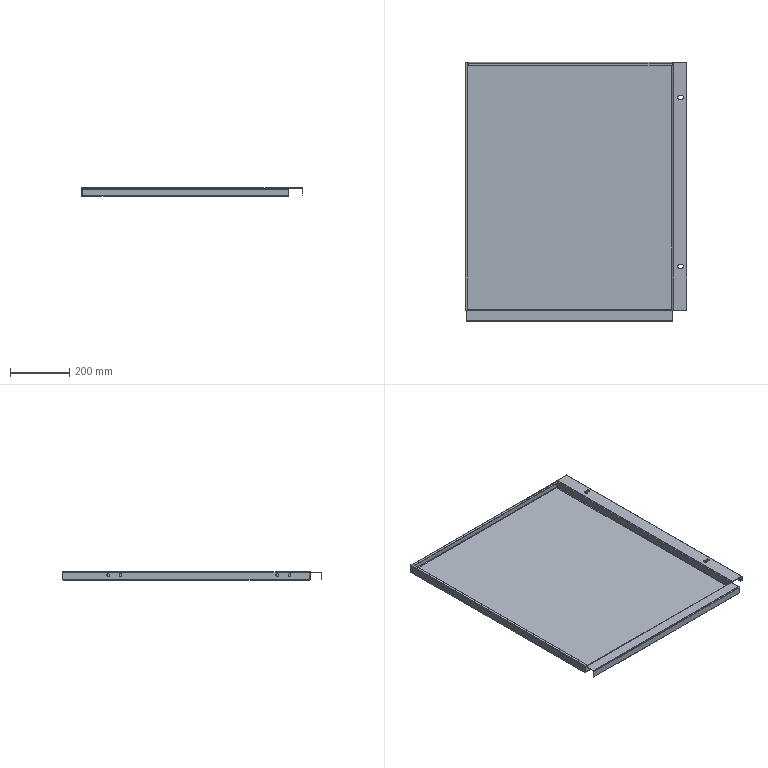Part | STEP file | Rear upper door (upper/lower interlock) | 1 solid | 119 faces | box 748.5 x 873.5 x 28 mm | volume 1158666 mm3 | plane 85 | cylinder 34 | commonest cylinder face diameters 3 x10 6 x10 9 x8 13 x6